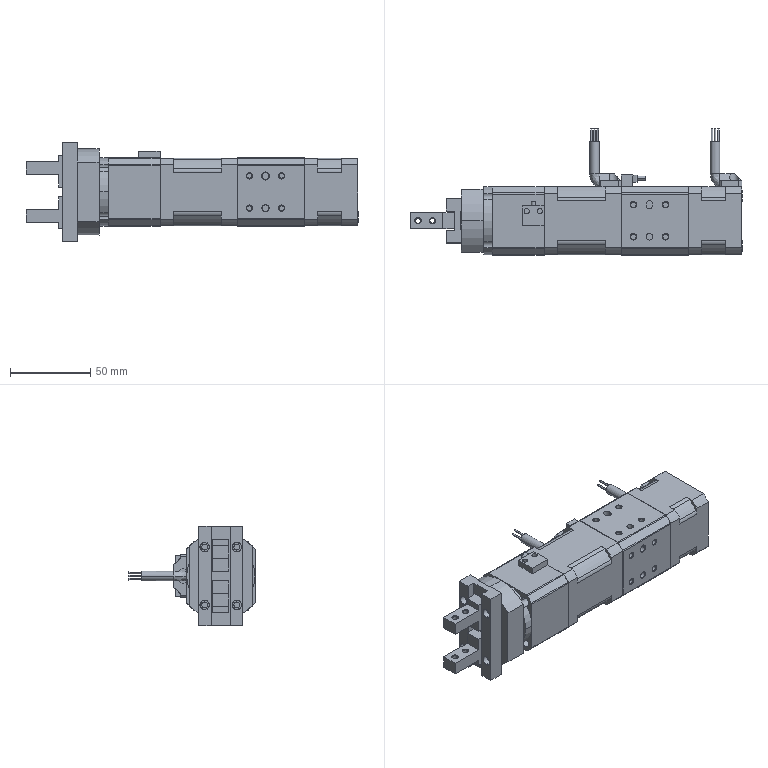Part | SolidWorks | 6 solids | 750 faces | box 206.7 x 78.5 x 62 mm | volume 306344 mm3 | cylinder 327 | plane 325 | cone 90 | spline 8 | commonest cylinder face diameters 3.2 x44 3.3 x32 2.5 x30 2 x28 54 x19 8 x18